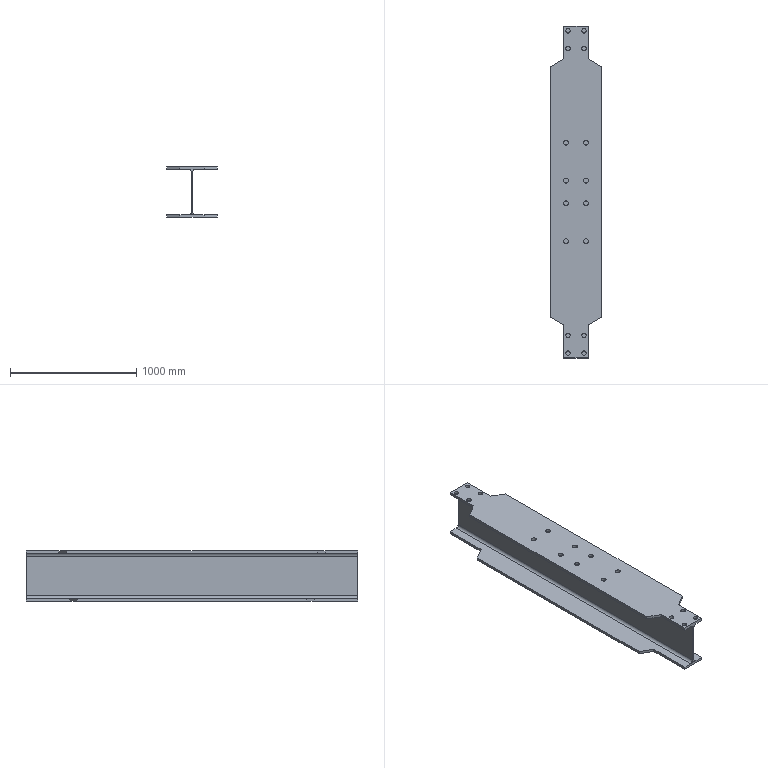Part | SolidWorks | features Cut 4, Extrusion 1 | 1 solid | 70 faces | box 400 x 2625 x 400 mm | volume 51162611 mm3 | cylinder 38 | plane 32 | commonest cylinder face diameters 35 x16 39 x16 44 x4 12.7 x2